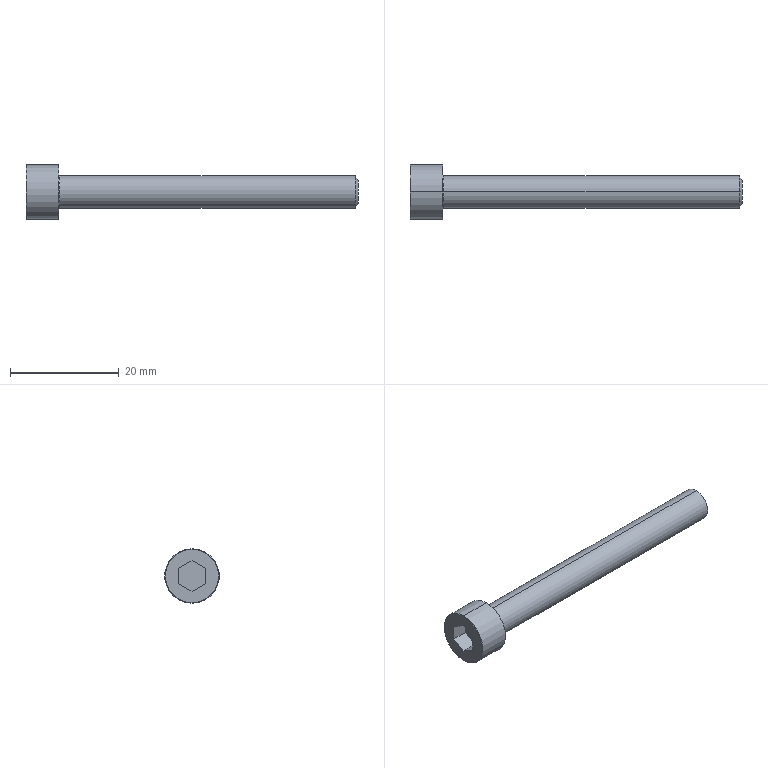Part | NX | features BREP 1 | 1 solid | 20 faces | box 61 x 10 x 10 mm | volume 1959 mm3 | plane 10 | torus 4 | cylinder 4 | cone 2 | commonest cylinder face diameters 6 x2 10 x2
STEP:
#1=CARTESIAN_POINT('',(0.,0.,4.9));
#2=VERTEX_POINT('',#1);
#3=CARTESIAN_POINT('',(0.,0.,-4.9));
#4=VERTEX_POINT('',#3);
#5=CARTESIAN_POINT('',(0.,0.,0.));
#6=DIRECTION('',(-1.,0.,0.));
#7=DIRECTION('',(0.,0.,-1.));
#8=AXIS2_PLACEMENT_3D('',#5,#6,#7);
#9=CIRCLE('',#8,4.9);
#10=EDGE_CURVE('',#2,#4,#9,.T.);
#11=ORIENTED_EDGE('',*,*,#10,.F.);
#12=CARTESIAN_POINT('',(0.1,0.,5.));
#13=VERTEX_POINT('',#12);
#14=CARTESIAN_POINT('',(0.1,0.,4.9));
#15=DIRECTION('',(0.,1.,0.));
#16=DIRECTION('',(0.,0.,1.));
#17=AXIS2_PLACEMENT_3D('',#14,#15,#16);
#18=CIRCLE('',#17,0.1);
#19=EDGE_CURVE('',#2,#13,#18,.T.);
#20=ORIENTED_EDGE('',*,*,#19,.T.);
#21=CARTESIAN_POINT('',(0.1,0.,-5.));
#22=VERTEX_POINT('',#21);
#23=CARTESIAN_POINT('',(0.1,0.,0.));
#24=DIRECTION('',(1.,0.,0.));
#25=DIRECTION('',(0.,0.,-1.));
#26=AXIS2_PLACEMENT_3D('',#23,#24,#25);
#27=CIRCLE('',#26,5.);
#28=EDGE_CURVE('',#22,#13,#27,.T.);
#29=ORIENTED_EDGE('',*,*,#28,.F.);
#30=CARTESIAN_POINT('',(0.1,0.,-4.9));
#31=DIRECTION('',(0.,-1.,0.));
#32=DIRECTION('',(0.,0.,-1.));
#33=AXIS2_PLACEMENT_3D('',#30,#31,#32);
#34=CIRCLE('',#33,0.1);
#35=EDGE_CURVE('',#4,#22,#34,.T.);
#36=ORIENTED_EDGE('',*,*,#35,.F.);
#37=EDGE_LOOP('',(#11,#20,#29,#36));
#38=FACE_BOUND('',#37,.T.);
#39=CARTESIAN_POINT('',(0.1,0.,0.));
#40=DIRECTION('',(1.,0.,0.));
#41=DIRECTION('',(0.,0.,-1.));
#42=AXIS2_PLACEMENT_3D('',#39,#40,#41);
#43=TOROIDAL_SURFACE('',#42,4.9,0.1);
#44=ADVANCED_FACE('',(#38),#43,.T.);
#45=CARTESIAN_POINT('',(61.,0.,2.134));
#46=VERTEX_POINT('',#45);
#47=CARTESIAN_POINT('',(61.,0.,-2.134));
#48=VERTEX_POINT('',#47);
#49=CARTESIAN_POINT('',(61.,0.,0.));
#50=DIRECTION('',(-1.,0.,0.));
#51=DIRECTION('',(0.,0.,1.));
#52=AXIS2_PLACEMENT_3D('',#49,#50,#51);
#53=CIRCLE('',#52,2.134);
#54=EDGE_CURVE('',#46,#48,#53,.T.);
#55=ORIENTED_EDGE('',*,*,#54,.T.);
#56=CARTESIAN_POINT('',(60.5,0.,-3.));
#57=VERTEX_POINT('',#56);
#58=CARTESIAN_POINT('',(60.5,0.,-3.));
#59=DIRECTION('',(-0.5,0.,-0.866));
#60=VECTOR('',#59,1000.);
#61=LINE('',#58,#60);
#62=EDGE_CURVE('',#57,#48,#61,.F.);
#63=ORIENTED_EDGE('',*,*,#62,.F.);
#64=CARTESIAN_POINT('',(60.5,0.,3.));
#65=VERTEX_POINT('',#64);
#66=CARTESIAN_POINT('',(60.5,0.,0.));
#67=DIRECTION('',(-1.,0.,0.));
#68=DIRECTION('',(0.,0.,1.));
#69=AXIS2_PLACEMENT_3D('',#66,#67,#68);
#70=CIRCLE('',#69,3.);
#71=EDGE_CURVE('',#65,#57,#70,.T.);
#72=ORIENTED_EDGE('',*,*,#71,.F.);
#73=CARTESIAN_POINT('',(60.5,0.,3.));
#74=DIRECTION('',(-0.5,0.,0.866));
#75=VECTOR('',#74,1000.);
#76=LINE('',#73,#75);
#77=EDGE_CURVE('',#65,#46,#76,.F.);
#78=ORIENTED_EDGE('',*,*,#77,.T.);
#79=EDGE_LOOP('',(#55,#63,#72,#78));
#80=FACE_BOUND('',#79,.T.);
#81=CARTESIAN_POINT('',(60.5,0.,0.));
#82=DIRECTION('',(-1.,0.,0.));
#83=DIRECTION('',(0.,0.,1.));
#84=AXIS2_PLACEMENT_3D('',#81,#82,#83);
#85=CONICAL_SURFACE('',#84,3.,1.047);
#86=ADVANCED_FACE('',(#80),#85,.T.);
#87=CARTESIAN_POINT('',(6.,0.,-3.2));
#88=VERTEX_POINT('',#87);
#89=CARTESIAN_POINT('',(6.,0.,3.2));
#90=VERTEX_POINT('',#89);
#91=CARTESIAN_POINT('',(6.,0.,0.));
#92=DIRECTION('',(-1.,0.,0.));
#93=DIRECTION('',(0.,0.,1.));
#94=AXIS2_PLACEMENT_3D('',#91,#92,#93);
#95=CIRCLE('',#94,3.2);
#96=EDGE_CURVE('',#88,#90,#95,.T.);
#97=ORIENTED_EDGE('',*,*,#96,.F.);
#98=CARTESIAN_POINT('',(6.2,0.,-3.));
#99=VERTEX_POINT('',#98);
#100=CARTESIAN_POINT('',(6.2,0.,-3.2));
#101=DIRECTION('',(0.,1.,0.));
#102=DIRECTION('',(0.,0.,1.));
#103=AXIS2_PLACEMENT_3D('',#100,#101,#102);
#104=CIRCLE('',#103,0.2);
#105=EDGE_CURVE('',#99,#88,#104,.F.);
#106=ORIENTED_EDGE('',*,*,#105,.F.);
#107=CARTESIAN_POINT('',(6.2,0.,3.));
#108=VERTEX_POINT('',#107);
#109=CARTESIAN_POINT('',(6.2,0.,0.));
#110=DIRECTION('',(-1.,0.,0.));
#111=DIRECTION('',(0.,0.,1.));
#112=AXIS2_PLACEMENT_3D('',#109,#110,#111);
#113=CIRCLE('',#112,3.);
#114=EDGE_CURVE('',#99,#108,#113,.T.);
#115=ORIENTED_EDGE('',*,*,#114,.T.);
#116=CARTESIAN_POINT('',(6.2,0.,3.2));
#117=DIRECTION('',(0.,-1.,0.));
#118=DIRECTION('',(0.,0.,-1.));
#119=AXIS2_PLACEMENT_3D('',#116,#117,#118);
#120=CIRCLE('',#119,0.2);
#121=EDGE_CURVE('',#108,#90,#120,.F.);
#122=ORIENTED_EDGE('',*,*,#121,.T.);
#123=EDGE_LOOP('',(#97,#106,#115,#122));
#124=FACE_BOUND('',#123,.T.);
#125=CARTESIAN_POINT('',(6.2,0.,0.));
#126=DIRECTION('',(-1.,0.,0.));
#127=DIRECTION('',(0.,0.,1.));
#128=AXIS2_PLACEMENT_3D('',#125,#126,#127);
#129=TOROIDAL_SURFACE('',#128,3.2,0.2);
#130=ADVANCED_FACE('',(#124),#129,.F.);
#131=CARTESIAN_POINT('',(6.,0.,5.));
#132=VERTEX_POINT('',#131);
#133=CARTESIAN_POINT('',(6.,0.,-5.));
#134=VERTEX_POINT('',#133);
#135=CARTESIAN_POINT('',(6.,0.,0.));
#136=DIRECTION('',(-1.,0.,0.));
#137=DIRECTION('',(0.,0.,1.));
#138=AXIS2_PLACEMENT_3D('',#135,#136,#137);
#139=CIRCLE('',#138,5.);
#140=EDGE_CURVE('',#132,#134,#139,.T.);
#141=ORIENTED_EDGE('',*,*,#140,.T.);
#142=CARTESIAN_POINT('',(0.,0.,-5.));
#143=DIRECTION('',(-1.,0.,0.));
#144=VECTOR('',#143,1000.);
#145=LINE('',#142,#144);
#146=EDGE_CURVE('',#22,#134,#145,.F.);
#147=ORIENTED_EDGE('',*,*,#146,.F.);
#148=ORIENTED_EDGE('',*,*,#28,.T.);
#149=CARTESIAN_POINT('',(0.,0.,5.));
#150=DIRECTION('',(-1.,0.,0.));
#151=VECTOR('',#150,1000.);
#152=LINE('',#149,#151);
#153=EDGE_CURVE('',#13,#132,#152,.F.);
#154=ORIENTED_EDGE('',*,*,#153,.T.);
#155=EDGE_LOOP('',(#141,#147,#148,#154));
#156=FACE_BOUND('',#155,.T.);
#157=CARTESIAN_POINT('',(0.,0.,0.));
#158=DIRECTION('',(-1.,0.,0.));
#159=DIRECTION('',(0.,0.,1.));
#160=AXIS2_PLACEMENT_3D('',#157,#158,#159);
#161=CYLINDRICAL_SURFACE('',#160,5.);
#162=ADVANCED_FACE('',(#156),#161,.T.);
#163=ORIENTED_EDGE('',*,*,#71,.T.);
#164=CARTESIAN_POINT('',(0.,0.,-3.));
#165=DIRECTION('',(-1.,0.,0.));
#166=VECTOR('',#165,1000.);
#167=LINE('',#164,#166);
#168=EDGE_CURVE('',#99,#57,#167,.F.);
#169=ORIENTED_EDGE('',*,*,#168,.F.);
#170=CARTESIAN_POINT('',(6.2,0.,0.));
#171=DIRECTION('',(-1.,0.,0.));
#172=DIRECTION('',(0.,0.,1.));
#173=AXIS2_PLACEMENT_3D('',#170,#171,#172);
#174=CIRCLE('',#173,3.);
#175=EDGE_CURVE('',#108,#99,#174,.T.);
#176=ORIENTED_EDGE('',*,*,#175,.F.);
#177=CARTESIAN_POINT('',(0.,0.,3.));
#178=DIRECTION('',(-1.,0.,0.));
#179=VECTOR('',#178,1000.);
#180=LINE('',#177,#179);
#181=EDGE_CURVE('',#108,#65,#180,.F.);
#182=ORIENTED_EDGE('',*,*,#181,.T.);
#183=EDGE_LOOP('',(#163,#169,#176,#182));
#184=FACE_BOUND('',#183,.T.);
#185=CARTESIAN_POINT('',(0.,0.,0.));
#186=DIRECTION('',(-1.,0.,0.));
#187=DIRECTION('',(0.,0.,1.));
#188=AXIS2_PLACEMENT_3D('',#185,#186,#187);
#189=CYLINDRICAL_SURFACE('',#188,3.);
#190=ADVANCED_FACE('',(#184),#189,.T.);
#191=ORIENTED_EDGE('',*,*,#168,.T.);
#192=CARTESIAN_POINT('',(60.5,0.,0.));
#193=DIRECTION('',(-1.,0.,0.));
#194=DIRECTION('',(0.,0.,1.));
#195=AXIS2_PLACEMENT_3D('',#192,#193,#194);
#196=CIRCLE('',#195,3.);
#197=EDGE_CURVE('',#57,#65,#196,.T.);
#198=ORIENTED_EDGE('',*,*,#197,.T.);
#199=ORIENTED_EDGE('',*,*,#181,.F.);
#200=ORIENTED_EDGE('',*,*,#114,.F.);
#201=EDGE_LOOP('',(#191,#198,#199,#200));
#202=FACE_BOUND('',#201,.T.);
#203=CARTESIAN_POINT('',(0.,0.,0.));
#204=DIRECTION('',(-1.,0.,0.));
#205=DIRECTION('',(0.,0.,1.));
#206=AXIS2_PLACEMENT_3D('',#203,#204,#205);
#207=CYLINDRICAL_SURFACE('',#206,3.);
#208=ADVANCED_FACE('',(#202),#207,.T.);
#209=CARTESIAN_POINT('',(0.,0.,0.));
#210=DIRECTION('',(-1.,0.,0.));
#211=DIRECTION('',(0.,0.,-1.));
#212=AXIS2_PLACEMENT_3D('',#209,#210,#211);
#213=CIRCLE('',#212,4.9);
#214=EDGE_CURVE('',#4,#2,#213,.T.);
#215=ORIENTED_EDGE('',*,*,#214,.T.);
#216=ORIENTED_EDGE('',*,*,#10,.T.);
#217=EDGE_LOOP('',(#215,#216));
#218=FACE_BOUND('',#217,.T.);
#219=CARTESIAN_POINT('',(0.,0.,2.86));
#220=VERTEX_POINT('',#219);
#221=CARTESIAN_POINT('',(0.,2.477,1.43));
#222=VERTEX_POINT('',#221);
#223=CARTESIAN_POINT('',(0.,0.,2.86));
#224=DIRECTION('',(0.,0.866,-0.5));
#225=VECTOR('',#224,1000.);
#226=LINE('',#223,#225);
#227=EDGE_CURVE('',#220,#222,#226,.T.);
#228=ORIENTED_EDGE('',*,*,#227,.F.);
#229=CARTESIAN_POINT('',(0.,-2.477,1.43));
#230=VERTEX_POINT('',#229);
#231=CARTESIAN_POINT('',(0.,-2.477,1.43));
#232=DIRECTION('',(0.,0.866,0.5));
#233=VECTOR('',#232,1000.);
#234=LINE('',#231,#233);
#235=EDGE_CURVE('',#230,#220,#234,.T.);
#236=ORIENTED_EDGE('',*,*,#235,.F.);
#237=CARTESIAN_POINT('',(0.,-2.477,-1.43));
#238=VERTEX_POINT('',#237);
#239=CARTESIAN_POINT('',(0.,-2.477,-1.43));
#240=DIRECTION('',(0.,0.,1.));
#241=VECTOR('',#240,1000.);
#242=LINE('',#239,#241);
#243=EDGE_CURVE('',#238,#230,#242,.T.);
#244=ORIENTED_EDGE('',*,*,#243,.F.);
#245=CARTESIAN_POINT('',(0.,0.,-2.86));
#246=VERTEX_POINT('',#245);
#247=CARTESIAN_POINT('',(0.,0.,-2.86));
#248=DIRECTION('',(0.,-0.866,0.5));
#249=VECTOR('',#248,1000.);
#250=LINE('',#247,#249);
#251=EDGE_CURVE('',#246,#238,#250,.T.);
#252=ORIENTED_EDGE('',*,*,#251,.F.);
#253=CARTESIAN_POINT('',(0.,2.477,-1.43));
#254=VERTEX_POINT('',#253);
#255=CARTESIAN_POINT('',(0.,2.477,-1.43));
#256=DIRECTION('',(0.,-0.866,-0.5));
#257=VECTOR('',#256,1000.);
#258=LINE('',#255,#257);
#259=EDGE_CURVE('',#254,#246,#258,.T.);
#260=ORIENTED_EDGE('',*,*,#259,.F.);
#261=CARTESIAN_POINT('',(0.,2.477,1.43));
#262=DIRECTION('',(0.,0.,-1.));
#263=VECTOR('',#262,1000.);
#264=LINE('',#261,#263);
#265=EDGE_CURVE('',#222,#254,#264,.T.);
#266=ORIENTED_EDGE('',*,*,#265,.F.);
#267=EDGE_LOOP('',(#228,#236,#244,#252,#260,#266));
#268=FACE_BOUND('',#267,.T.);
#269=CARTESIAN_POINT('',(0.,0.,0.));
#270=DIRECTION('',(1.,0.,0.));
#271=DIRECTION('',(0.,1.,0.));
#272=AXIS2_PLACEMENT_3D('',#269,#270,#271);
#273=PLANE('',#272);
#274=ADVANCED_FACE('',(#218,#268),#273,.F.);
#275=ORIENTED_EDGE('',*,*,#146,.T.);
#276=CARTESIAN_POINT('',(6.,0.,0.));
#277=DIRECTION('',(-1.,0.,0.));
#278=DIRECTION('',(0.,0.,1.));
#279=AXIS2_PLACEMENT_3D('',#276,#277,#278);
#280=CIRCLE('',#279,5.);
#281=EDGE_CURVE('',#134,#132,#280,.T.);
#282=ORIENTED_EDGE('',*,*,#281,.T.);
#283=ORIENTED_EDGE('',*,*,#153,.F.);
#284=CARTESIAN_POINT('',(0.1,0.,0.));
#285=DIRECTION('',(1.,0.,0.));
#286=DIRECTION('',(0.,0.,-1.));
#287=AXIS2_PLACEMENT_3D('',#284,#285,#286);
#288=CIRCLE('',#287,5.);
#289=EDGE_CURVE('',#13,#22,#288,.T.);
#290=ORIENTED_EDGE('',*,*,#289,.T.);
#291=EDGE_LOOP('',(#275,#282,#283,#290));
#292=FACE_BOUND('',#291,.T.);
#293=CARTESIAN_POINT('',(0.,0.,0.));
#294=DIRECTION('',(-1.,0.,0.));
#295=DIRECTION('',(0.,0.,1.));
#296=AXIS2_PLACEMENT_3D('',#293,#294,#295);
#297=CYLINDRICAL_SURFACE('',#296,5.);
#298=ADVANCED_FACE('',(#292),#297,.T.);
#299=ORIENTED_EDGE('',*,*,#140,.F.);
#300=ORIENTED_EDGE('',*,*,#281,.F.);
#301=EDGE_LOOP('',(#299,#300));
#302=FACE_BOUND('',#301,.T.);
#303=CARTESIAN_POINT('',(6.,0.,0.));
#304=DIRECTION('',(-1.,0.,0.));
#305=DIRECTION('',(0.,0.,1.));
#306=AXIS2_PLACEMENT_3D('',#303,#304,#305);
#307=CIRCLE('',#306,3.2);
#308=EDGE_CURVE('',#90,#88,#307,.T.);
#309=ORIENTED_EDGE('',*,*,#308,.T.);
#310=ORIENTED_EDGE('',*,*,#96,.T.);
#311=EDGE_LOOP('',(#309,#310));
#312=FACE_BOUND('',#311,.T.);
#313=CARTESIAN_POINT('',(6.,5.,0.));
#314=DIRECTION('',(-1.,0.,0.));
#315=DIRECTION('',(0.,0.,1.));
#316=AXIS2_PLACEMENT_3D('',#313,#314,#315);
#317=PLANE('',#316);
#318=ADVANCED_FACE('',(#302,#312),#317,.F.);
#319=ORIENTED_EDGE('',*,*,#105,.T.);
#320=ORIENTED_EDGE('',*,*,#308,.F.);
#321=ORIENTED_EDGE('',*,*,#121,.F.);
#322=ORIENTED_EDGE('',*,*,#175,.T.);
#323=EDGE_LOOP('',(#319,#320,#321,#322));
#324=FACE_BOUND('',#323,.T.);
#325=CARTESIAN_POINT('',(6.2,0.,0.));
#326=DIRECTION('',(-1.,0.,0.));
#327=DIRECTION('',(0.,0.,1.));
#328=AXIS2_PLACEMENT_3D('',#325,#326,#327);
#329=TOROIDAL_SURFACE('',#328,3.2,0.2);
#330=ADVANCED_FACE('',(#324),#329,.F.);
#331=ORIENTED_EDGE('',*,*,#235,.T.);
#332=CARTESIAN_POINT('',(3.,0.,2.86));
#333=VERTEX_POINT('',#332);
#334=CARTESIAN_POINT('',(3.,0.,2.86));
#335=DIRECTION('',(-1.,0.,0.));
#336=VECTOR('',#335,1000.);
#337=LINE('',#334,#336);
#338=EDGE_CURVE('',#333,#220,#337,.T.);
#339=ORIENTED_EDGE('',*,*,#338,.F.);
#340=CARTESIAN_POINT('',(3.,-2.477,1.43));
#341=VERTEX_POINT('',#340);
#342=CARTESIAN_POINT('',(3.,-2.477,1.43));
#343=DIRECTION('',(0.,0.866,0.5));
#344=VECTOR('',#343,1000.);
#345=LINE('',#342,#344);
#346=EDGE_CURVE('',#341,#333,#345,.T.);
#347=ORIENTED_EDGE('',*,*,#346,.F.);
#348=CARTESIAN_POINT('',(3.,-2.477,1.43));
#349=DIRECTION('',(-1.,0.,0.));
#350=VECTOR('',#349,1000.);
#351=LINE('',#348,#350);
#352=EDGE_CURVE('',#341,#230,#351,.T.);
#353=ORIENTED_EDGE('',*,*,#352,.T.);
#354=EDGE_LOOP('',(#331,#339,#347,#353));
#355=FACE_BOUND('',#354,.T.);
#356=CARTESIAN_POINT('',(3.,-2.477,1.43));
#357=DIRECTION('',(0.,-0.5,0.866));
#358=DIRECTION('',(-1.,0.,0.));
#359=AXIS2_PLACEMENT_3D('',#356,#357,#358);
#360=PLANE('',#359);
#361=ADVANCED_FACE('',(#355),#360,.F.);
#362=ORIENTED_EDGE('',*,*,#243,.T.);
#363=ORIENTED_EDGE('',*,*,#352,.F.);
#364=CARTESIAN_POINT('',(3.,-2.477,-1.43));
#365=VERTEX_POINT('',#364);
#366=CARTESIAN_POINT('',(3.,-2.477,-1.43));
#367=DIRECTION('',(0.,0.,1.));
#368=VECTOR('',#367,1000.);
#369=LINE('',#366,#368);
#370=EDGE_CURVE('',#365,#341,#369,.T.);
#371=ORIENTED_EDGE('',*,*,#370,.F.);
#372=CARTESIAN_POINT('',(3.,-2.477,-1.43));
#373=DIRECTION('',(-1.,0.,0.));
#374=VECTOR('',#373,1000.);
#375=LINE('',#372,#374);
#376=EDGE_CURVE('',#365,#238,#375,.T.);
#377=ORIENTED_EDGE('',*,*,#376,.T.);
#378=EDGE_LOOP('',(#362,#363,#371,#377));
#379=FACE_BOUND('',#378,.T.);
#380=CARTESIAN_POINT('',(3.,-2.477,-1.43));
#381=DIRECTION('',(0.,-1.,0.));
#382=DIRECTION('',(0.,0.,-1.));
#383=AXIS2_PLACEMENT_3D('',#380,#381,#382);
#384=PLANE('',#383);
#385=ADVANCED_FACE('',(#379),#384,.F.);
#386=ORIENTED_EDGE('',*,*,#251,.T.);
#387=ORIENTED_EDGE('',*,*,#376,.F.);
#388=CARTESIAN_POINT('',(3.,0.,-2.86));
#389=VERTEX_POINT('',#388);
#390=CARTESIAN_POINT('',(3.,0.,-2.86));
#391=DIRECTION('',(0.,-0.866,0.5));
#392=VECTOR('',#391,1000.);
#393=LINE('',#390,#392);
#394=EDGE_CURVE('',#389,#365,#393,.T.);
#395=ORIENTED_EDGE('',*,*,#394,.F.);
#396=CARTESIAN_POINT('',(3.,0.,-2.86));
#397=DIRECTION('',(-1.,0.,0.));
#398=VECTOR('',#397,1000.);
#399=LINE('',#396,#398);
#400=EDGE_CURVE('',#389,#246,#399,.T.);
#401=ORIENTED_EDGE('',*,*,#400,.T.);
#402=EDGE_LOOP('',(#386,#387,#395,#401));
#403=FACE_BOUND('',#402,.T.);
#404=CARTESIAN_POINT('',(3.,0.,-2.86));
#405=DIRECTION('',(0.,-0.5,-0.866));
#406=DIRECTION('',(0.,-0.866,0.5));
#407=AXIS2_PLACEMENT_3D('',#404,#405,#406);
#408=PLANE('',#407);
#409=ADVANCED_FACE('',(#403),#408,.F.);
#410=ORIENTED_EDGE('',*,*,#259,.T.);
#411=ORIENTED_EDGE('',*,*,#400,.F.);
#412=CARTESIAN_POINT('',(3.,2.477,-1.43));
#413=VERTEX_POINT('',#412);
#414=CARTESIAN_POINT('',(3.,2.477,-1.43));
#415=DIRECTION('',(0.,-0.866,-0.5));
#416=VECTOR('',#415,1000.);
#417=LINE('',#414,#416);
#418=EDGE_CURVE('',#413,#389,#417,.T.);
#419=ORIENTED_EDGE('',*,*,#418,.F.);
#420=CARTESIAN_POINT('',(3.,2.477,-1.43));
#421=DIRECTION('',(-1.,0.,0.));
#422=VECTOR('',#421,1000.);
#423=LINE('',#420,#422);
#424=EDGE_CURVE('',#413,#254,#423,.T.);
#425=ORIENTED_EDGE('',*,*,#424,.T.);
#426=EDGE_LOOP('',(#410,#411,#419,#425));
#427=FACE_BOUND('',#426,.T.);
#428=CARTESIAN_POINT('',(3.,2.477,-1.43));
#429=DIRECTION('',(0.,0.5,-0.866));
#430=DIRECTION('',(-1.,0.,0.));
#431=AXIS2_PLACEMENT_3D('',#428,#429,#430);
#432=PLANE('',#431);
#433=ADVANCED_FACE('',(#427),#432,.F.);
#434=ORIENTED_EDGE('',*,*,#265,.T.);
#435=ORIENTED_EDGE('',*,*,#424,.F.);
#436=CARTESIAN_POINT('',(3.,2.477,1.43));
#437=VERTEX_POINT('',#436);
#438=CARTESIAN_POINT('',(3.,2.477,1.43));
#439=DIRECTION('',(0.,0.,-1.));
#440=VECTOR('',#439,1000.);
#441=LINE('',#438,#440);
#442=EDGE_CURVE('',#437,#413,#441,.T.);
#443=ORIENTED_EDGE('',*,*,#442,.F.);
#444=CARTESIAN_POINT('',(3.,2.477,1.43));
#445=DIRECTION('',(-1.,0.,0.));
#446=VECTOR('',#445,1000.);
#447=LINE('',#444,#446);
#448=EDGE_CURVE('',#437,#222,#447,.T.);
#449=ORIENTED_EDGE('',*,*,#448,.T.);
#450=EDGE_LOOP('',(#434,#435,#443,#449));
#451=FACE_BOUND('',#450,.T.);
#452=CARTESIAN_POINT('',(3.,2.477,1.43));
#453=DIRECTION('',(0.,1.,0.));
#454=DIRECTION('',(1.,0.,0.));
#455=AXIS2_PLACEMENT_3D('',#452,#453,#454);
#456=PLANE('',#455);
#457=ADVANCED_FACE('',(#451),#456,.F.);
#458=ORIENTED_EDGE('',*,*,#227,.T.);
#459=ORIENTED_EDGE('',*,*,#448,.F.);
#460=CARTESIAN_POINT('',(3.,0.,2.86));
#461=DIRECTION('',(0.,0.866,-0.5));
#462=VECTOR('',#461,1000.);
#463=LINE('',#460,#462);
#464=EDGE_CURVE('',#333,#437,#463,.T.);
#465=ORIENTED_EDGE('',*,*,#464,.F.);
#466=ORIENTED_EDGE('',*,*,#338,.T.);
#467=EDGE_LOOP('',(#458,#459,#465,#466));
#468=FACE_BOUND('',#467,.T.);
#469=CARTESIAN_POINT('',(3.,0.,2.86));
#470=DIRECTION('',(0.,0.5,0.866));
#471=DIRECTION('',(1.,0.,0.));
#472=AXIS2_PLACEMENT_3D('',#469,#470,#471);
#473=PLANE('',#472);
#474=ADVANCED_FACE('',(#468),#473,.F.);
#475=ORIENTED_EDGE('',*,*,#346,.T.);
#476=ORIENTED_EDGE('',*,*,#464,.T.);
#477=ORIENTED_EDGE('',*,*,#442,.T.);
#478=ORIENTED_EDGE('',*,*,#418,.T.);
#479=ORIENTED_EDGE('',*,*,#394,.T.);
#480=ORIENTED_EDGE('',*,*,#370,.T.);
#481=EDGE_LOOP('',(#475,#476,#477,#478,#479,#480));
#482=FACE_BOUND('',#481,.T.);
#483=CARTESIAN_POINT('',(3.,-2.477,1.43));
#484=DIRECTION('',(1.,0.,0.));
#485=DIRECTION('',(0.,1.,0.));
#486=AXIS2_PLACEMENT_3D('',#483,#484,#485);
#487=PLANE('',#486);
#488=ADVANCED_FACE('',(#482),#487,.F.);
#489=ORIENTED_EDGE('',*,*,#62,.T.);
#490=CARTESIAN_POINT('',(61.,0.,0.));
#491=DIRECTION('',(-1.,0.,0.));
#492=DIRECTION('',(0.,0.,1.));
#493=AXIS2_PLACEMENT_3D('',#490,#491,#492);
#494=CIRCLE('',#493,2.134);
#495=EDGE_CURVE('',#48,#46,#494,.T.);
#496=ORIENTED_EDGE('',*,*,#495,.T.);
#497=ORIENTED_EDGE('',*,*,#77,.F.);
#498=ORIENTED_EDGE('',*,*,#197,.F.);
#499=EDGE_LOOP('',(#489,#496,#497,#498));
#500=FACE_BOUND('',#499,.T.);
#501=CARTESIAN_POINT('',(60.5,0.,0.));
#502=DIRECTION('',(-1.,0.,0.));
#503=DIRECTION('',(0.,0.,1.));
#504=AXIS2_PLACEMENT_3D('',#501,#502,#503);
#505=CONICAL_SURFACE('',#504,3.,1.047);
#506=ADVANCED_FACE('',(#500),#505,.T.);
#507=ORIENTED_EDGE('',*,*,#54,.F.);
#508=ORIENTED_EDGE('',*,*,#495,.F.);
#509=EDGE_LOOP('',(#507,#508));
#510=FACE_BOUND('',#509,.T.);
#511=CARTESIAN_POINT('',(61.,3.,0.));
#512=DIRECTION('',(-1.,0.,0.));
#513=DIRECTION('',(0.,0.,1.));
#514=AXIS2_PLACEMENT_3D('',#511,#512,#513);
#515=PLANE('',#514);
#516=ADVANCED_FACE('',(#510),#515,.F.);
#517=ORIENTED_EDGE('',*,*,#19,.F.);
#518=ORIENTED_EDGE('',*,*,#214,.F.);
#519=ORIENTED_EDGE('',*,*,#35,.T.);
#520=ORIENTED_EDGE('',*,*,#289,.F.);
#521=EDGE_LOOP('',(#517,#518,#519,#520));
#522=FACE_BOUND('',#521,.T.);
#523=CARTESIAN_POINT('',(0.1,0.,0.));
#524=DIRECTION('',(1.,0.,0.));
#525=DIRECTION('',(0.,0.,-1.));
#526=AXIS2_PLACEMENT_3D('',#523,#524,#525);
#527=TOROIDAL_SURFACE('',#526,4.9,0.1);
#528=ADVANCED_FACE('',(#522),#527,.T.);
#529=CLOSED_SHELL('',(#44,#86,#130,#162,#190,#208,#274,#298,#318,#330,#361,#385,#409,#433,#457,#474,#488,#506,#516,#528));
#530=MANIFOLD_SOLID_BREP('',#529);
#531=(LENGTH_UNIT()NAMED_UNIT(*)SI_UNIT(.MILLI.,.METRE.));
#532=UNCERTAINTY_MEASURE_WITH_UNIT(LENGTH_MEASURE(0.00001),#531,'','');
#533=(NAMED_UNIT(*)PLANE_ANGLE_UNIT()SI_UNIT($,.RADIAN.));
#534=(NAMED_UNIT(*)SI_UNIT($,.STERADIAN.)SOLID_ANGLE_UNIT());
#535=(GEOMETRIC_REPRESENTATION_CONTEXT(3)GLOBAL_UNCERTAINTY_ASSIGNED_CONTEXT((#532))GLOBAL_UNIT_ASSIGNED_CONTEXT((#531,#533,#534))REPRESENTATION_CONTEXT('',''));
#536=ADVANCED_BREP_SHAPE_REPRESENTATION('',(#530),#535);